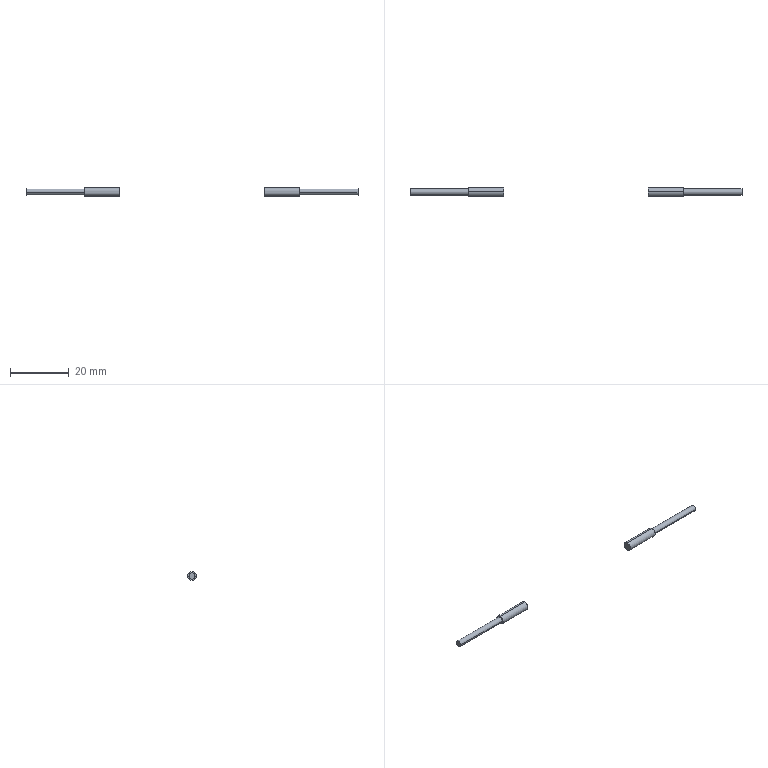Part | NX | 2 solids | 14 faces | box 113.5 x 3 x 3 mm | volume 308.19 mm3 | cylinder 8 | plane 6 | commonest cylinder face diameters 2.1 x4 3 x4